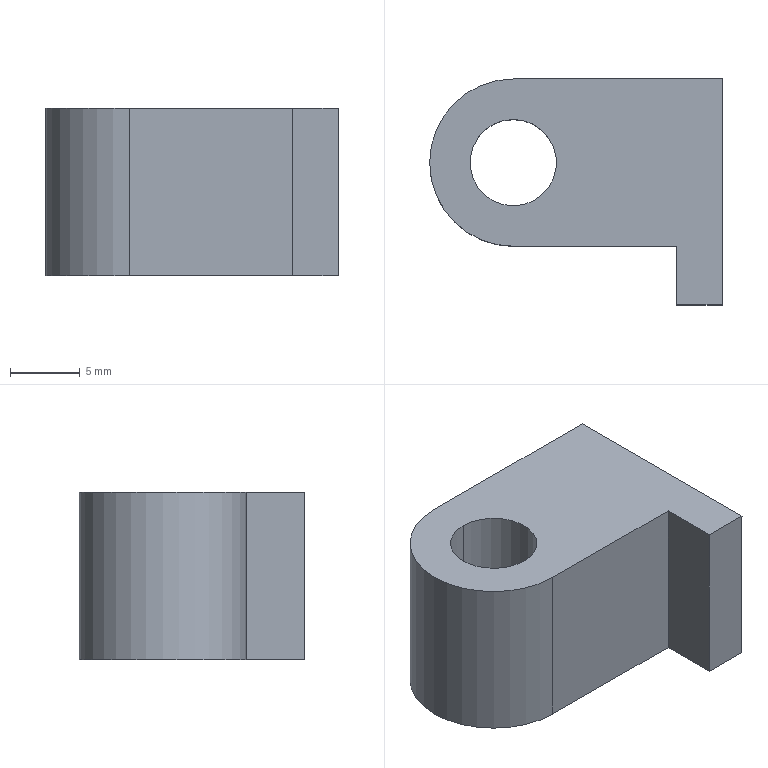Part | SolidWorks | features BaseBody 1 | 1 solid | 13 faces | box 21 x 16.2 x 12 mm | volume 2422 mm3 | plane 8 | cylinder 5 | commonest cylinder face diameters 5.3 x2 6.2 x2 12 x1
STEP:
#1=CARTESIAN_POINT('',(0.,-3.1,12.));
#2=VERTEX_POINT('',#1);
#3=CARTESIAN_POINT('',(0.,3.1,12.));
#4=VERTEX_POINT('',#3);
#5=CARTESIAN_POINT('',(0.,0.,12.));
#6=DIRECTION('',(0.,0.,-1.));
#7=DIRECTION('',(0.,1.,0.));
#8=AXIS2_PLACEMENT_3D('',#5,#6,#7);
#9=CIRCLE('',#8,3.1);
#10=EDGE_CURVE('',#2,#4,#9,.T.);
#11=ORIENTED_EDGE('',*,*,#10,.F.);
#12=CARTESIAN_POINT('',(0.,-3.1,0.));
#13=VERTEX_POINT('',#12);
#14=CARTESIAN_POINT('',(0.,-3.1,12.));
#15=DIRECTION('',(0.,0.,-1.));
#16=VECTOR('',#15,1000.);
#17=LINE('',#14,#16);
#18=EDGE_CURVE('',#2,#13,#17,.T.);
#19=ORIENTED_EDGE('',*,*,#18,.T.);
#20=CARTESIAN_POINT('',(0.,3.1,0.));
#21=VERTEX_POINT('',#20);
#22=CARTESIAN_POINT('',(0.,0.,0.));
#23=DIRECTION('',(0.,0.,1.));
#24=DIRECTION('',(0.,1.,0.));
#25=AXIS2_PLACEMENT_3D('',#22,#23,#24);
#26=CIRCLE('',#25,3.1);
#27=EDGE_CURVE('',#21,#13,#26,.T.);
#28=ORIENTED_EDGE('',*,*,#27,.F.);
#29=CARTESIAN_POINT('',(0.,3.1,12.));
#30=DIRECTION('',(0.,0.,-1.));
#31=VECTOR('',#30,1000.);
#32=LINE('',#29,#31);
#33=EDGE_CURVE('',#4,#21,#32,.T.);
#34=ORIENTED_EDGE('',*,*,#33,.F.);
#35=EDGE_LOOP('',(#11,#19,#28,#34));
#36=FACE_OUTER_BOUND('',#35,.T.);
#37=CARTESIAN_POINT('',(0.,0.,12.));
#38=DIRECTION('',(0.,0.,-1.));
#39=DIRECTION('',(0.,1.,0.));
#40=AXIS2_PLACEMENT_3D('',#37,#38,#39);
#41=CYLINDRICAL_SURFACE('',#40,3.1);
#42=ADVANCED_FACE('',(#36),#41,.F.);
#43=CARTESIAN_POINT('',(5.,-4.75,6.));
#44=VERTEX_POINT('',#43);
#45=CARTESIAN_POINT('',(5.,0.55,6.));
#46=VERTEX_POINT('',#45);
#47=CARTESIAN_POINT('',(5.,-2.1,6.));
#48=DIRECTION('',(1.,0.,0.));
#49=DIRECTION('',(0.,1.,0.));
#50=AXIS2_PLACEMENT_3D('',#47,#48,#49);
#51=CIRCLE('',#50,2.65);
#52=EDGE_CURVE('',#44,#46,#51,.T.);
#53=ORIENTED_EDGE('',*,*,#52,.F.);
#54=CARTESIAN_POINT('',(15.,-4.75,6.));
#55=VERTEX_POINT('',#54);
#56=CARTESIAN_POINT('',(5.,-4.75,6.));
#57=DIRECTION('',(1.,0.,0.));
#58=VECTOR('',#57,1000.);
#59=LINE('',#56,#58);
#60=EDGE_CURVE('',#44,#55,#59,.T.);
#61=ORIENTED_EDGE('',*,*,#60,.T.);
#62=CARTESIAN_POINT('',(15.,0.55,6.));
#63=VERTEX_POINT('',#62);
#64=CARTESIAN_POINT('',(15.,-2.1,6.));
#65=DIRECTION('',(1.,0.,0.));
#66=DIRECTION('',(0.,1.,0.));
#67=AXIS2_PLACEMENT_3D('',#64,#65,#66);
#68=CIRCLE('',#67,2.65);
#69=EDGE_CURVE('',#55,#63,#68,.T.);
#70=ORIENTED_EDGE('',*,*,#69,.T.);
#71=CARTESIAN_POINT('',(5.,0.55,6.));
#72=DIRECTION('',(1.,0.,0.));
#73=VECTOR('',#72,1000.);
#74=LINE('',#71,#73);
#75=EDGE_CURVE('',#46,#63,#74,.T.);
#76=ORIENTED_EDGE('',*,*,#75,.F.);
#77=EDGE_LOOP('',(#53,#61,#70,#76));
#78=FACE_OUTER_BOUND('',#77,.T.);
#79=CARTESIAN_POINT('',(5.,-2.1,6.));
#80=DIRECTION('',(1.,0.,0.));
#81=DIRECTION('',(0.,1.,0.));
#82=AXIS2_PLACEMENT_3D('',#79,#80,#81);
#83=CYLINDRICAL_SURFACE('',#82,2.65);
#84=ADVANCED_FACE('',(#78),#83,.F.);
#85=CARTESIAN_POINT('',(0.,0.,12.));
#86=DIRECTION('',(0.,0.,-1.));
#87=DIRECTION('',(0.,1.,0.));
#88=AXIS2_PLACEMENT_3D('',#85,#86,#87);
#89=CIRCLE('',#88,3.1);
#90=EDGE_CURVE('',#4,#2,#89,.T.);
#91=ORIENTED_EDGE('',*,*,#90,.T.);
#92=ORIENTED_EDGE('',*,*,#10,.T.);
#93=EDGE_LOOP('',(#91,#92));
#94=FACE_BOUND('',#93,.T.);
#95=CARTESIAN_POINT('',(15.,-10.2,12.));
#96=VERTEX_POINT('',#95);
#97=CARTESIAN_POINT('',(15.,6.,12.));
#98=VERTEX_POINT('',#97);
#99=CARTESIAN_POINT('',(15.,0.,12.));
#100=DIRECTION('',(0.,1.,0.));
#101=VECTOR('',#100,1000.);
#102=LINE('',#99,#101);
#103=EDGE_CURVE('',#96,#98,#102,.T.);
#104=ORIENTED_EDGE('',*,*,#103,.T.);
#105=CARTESIAN_POINT('',(0.,6.,12.));
#106=VERTEX_POINT('',#105);
#107=CARTESIAN_POINT('',(0.,6.,12.));
#108=DIRECTION('',(-1.,0.,0.));
#109=VECTOR('',#108,1000.);
#110=LINE('',#107,#109);
#111=EDGE_CURVE('',#98,#106,#110,.T.);
#112=ORIENTED_EDGE('',*,*,#111,.T.);
#113=CARTESIAN_POINT('',(0.,-6.,12.));
#114=VERTEX_POINT('',#113);
#115=CARTESIAN_POINT('',(0.,0.,12.));
#116=DIRECTION('',(0.,0.,1.));
#117=DIRECTION('',(0.,1.,0.));
#118=AXIS2_PLACEMENT_3D('',#115,#116,#117);
#119=CIRCLE('',#118,6.);
#120=EDGE_CURVE('',#106,#114,#119,.T.);
#121=ORIENTED_EDGE('',*,*,#120,.T.);
#122=CARTESIAN_POINT('',(11.7,-6.,12.));
#123=VERTEX_POINT('',#122);
#124=CARTESIAN_POINT('',(0.,-6.,12.));
#125=DIRECTION('',(1.,0.,0.));
#126=VECTOR('',#125,1000.);
#127=LINE('',#124,#126);
#128=EDGE_CURVE('',#114,#123,#127,.T.);
#129=ORIENTED_EDGE('',*,*,#128,.T.);
#130=CARTESIAN_POINT('',(11.7,-10.2,12.));
#131=VERTEX_POINT('',#130);
#132=CARTESIAN_POINT('',(11.7,0.,12.));
#133=DIRECTION('',(0.,-1.,0.));
#134=VECTOR('',#133,1000.);
#135=LINE('',#132,#134);
#136=EDGE_CURVE('',#123,#131,#135,.T.);
#137=ORIENTED_EDGE('',*,*,#136,.T.);
#138=CARTESIAN_POINT('',(0.,-10.2,12.));
#139=DIRECTION('',(1.,0.,0.));
#140=VECTOR('',#139,1000.);
#141=LINE('',#138,#140);
#142=EDGE_CURVE('',#131,#96,#141,.T.);
#143=ORIENTED_EDGE('',*,*,#142,.T.);
#144=EDGE_LOOP('',(#104,#112,#121,#129,#137,#143));
#145=FACE_OUTER_BOUND('',#144,.T.);
#146=CARTESIAN_POINT('',(0.,0.,12.));
#147=DIRECTION('',(0.,0.,1.));
#148=DIRECTION('',(0.,-1.,0.));
#149=AXIS2_PLACEMENT_3D('',#146,#147,#148);
#150=PLANE('',#149);
#151=ADVANCED_FACE('',(#94,#145),#150,.T.);
#152=ORIENTED_EDGE('',*,*,#18,.F.);
#153=ORIENTED_EDGE('',*,*,#90,.F.);
#154=ORIENTED_EDGE('',*,*,#33,.T.);
#155=CARTESIAN_POINT('',(0.,0.,0.));
#156=DIRECTION('',(0.,0.,1.));
#157=DIRECTION('',(0.,1.,0.));
#158=AXIS2_PLACEMENT_3D('',#155,#156,#157);
#159=CIRCLE('',#158,3.1);
#160=EDGE_CURVE('',#13,#21,#159,.T.);
#161=ORIENTED_EDGE('',*,*,#160,.F.);
#162=EDGE_LOOP('',(#152,#153,#154,#161));
#163=FACE_OUTER_BOUND('',#162,.T.);
#164=CARTESIAN_POINT('',(0.,0.,12.));
#165=DIRECTION('',(0.,0.,-1.));
#166=DIRECTION('',(0.,1.,0.));
#167=AXIS2_PLACEMENT_3D('',#164,#165,#166);
#168=CYLINDRICAL_SURFACE('',#167,3.1);
#169=ADVANCED_FACE('',(#163),#168,.F.);
#170=CARTESIAN_POINT('',(0.,6.,0.));
#171=VERTEX_POINT('',#170);
#172=CARTESIAN_POINT('',(0.,6.,12.));
#173=DIRECTION('',(0.,0.,-1.));
#174=VECTOR('',#173,1000.);
#175=LINE('',#172,#174);
#176=EDGE_CURVE('',#106,#171,#175,.T.);
#177=ORIENTED_EDGE('',*,*,#176,.F.);
#178=ORIENTED_EDGE('',*,*,#111,.F.);
#179=CARTESIAN_POINT('',(15.,6.,0.));
#180=VERTEX_POINT('',#179);
#181=CARTESIAN_POINT('',(15.,6.,12.));
#182=DIRECTION('',(0.,0.,1.));
#183=VECTOR('',#182,1000.);
#184=LINE('',#181,#183);
#185=EDGE_CURVE('',#180,#98,#184,.T.);
#186=ORIENTED_EDGE('',*,*,#185,.F.);
#187=CARTESIAN_POINT('',(0.,6.,0.));
#188=DIRECTION('',(1.,0.,0.));
#189=VECTOR('',#188,1000.);
#190=LINE('',#187,#189);
#191=EDGE_CURVE('',#171,#180,#190,.T.);
#192=ORIENTED_EDGE('',*,*,#191,.F.);
#193=EDGE_LOOP('',(#177,#178,#186,#192));
#194=FACE_OUTER_BOUND('',#193,.T.);
#195=CARTESIAN_POINT('',(0.,6.,12.));
#196=DIRECTION('',(0.,-1.,0.));
#197=DIRECTION('',(1.,0.,0.));
#198=AXIS2_PLACEMENT_3D('',#195,#196,#197);
#199=PLANE('',#198);
#200=ADVANCED_FACE('',(#194),#199,.F.);
#201=ORIENTED_EDGE('',*,*,#185,.T.);
#202=ORIENTED_EDGE('',*,*,#103,.F.);
#203=CARTESIAN_POINT('',(15.,-10.2,0.));
#204=VERTEX_POINT('',#203);
#205=CARTESIAN_POINT('',(15.,-10.2,12.));
#206=DIRECTION('',(0.,0.,1.));
#207=VECTOR('',#206,1000.);
#208=LINE('',#205,#207);
#209=EDGE_CURVE('',#204,#96,#208,.T.);
#210=ORIENTED_EDGE('',*,*,#209,.F.);
#211=CARTESIAN_POINT('',(15.,6.,0.));
#212=DIRECTION('',(0.,-1.,0.));
#213=VECTOR('',#212,1000.);
#214=LINE('',#211,#213);
#215=EDGE_CURVE('',#180,#204,#214,.T.);
#216=ORIENTED_EDGE('',*,*,#215,.F.);
#217=EDGE_LOOP('',(#201,#202,#210,#216));
#218=FACE_OUTER_BOUND('',#217,.T.);
#219=CARTESIAN_POINT('',(15.,-2.1,6.));
#220=DIRECTION('',(1.,0.,0.));
#221=DIRECTION('',(0.,1.,0.));
#222=AXIS2_PLACEMENT_3D('',#219,#220,#221);
#223=CIRCLE('',#222,2.65);
#224=EDGE_CURVE('',#63,#55,#223,.T.);
#225=ORIENTED_EDGE('',*,*,#224,.F.);
#226=ORIENTED_EDGE('',*,*,#69,.F.);
#227=EDGE_LOOP('',(#225,#226));
#228=FACE_BOUND('',#227,.T.);
#229=CARTESIAN_POINT('',(15.,6.,12.));
#230=DIRECTION('',(-1.,0.,0.));
#231=DIRECTION('',(0.,-1.,0.));
#232=AXIS2_PLACEMENT_3D('',#229,#230,#231);
#233=PLANE('',#232);
#234=ADVANCED_FACE('',(#218,#228),#233,.F.);
#235=ORIENTED_EDGE('',*,*,#209,.T.);
#236=ORIENTED_EDGE('',*,*,#142,.F.);
#237=CARTESIAN_POINT('',(11.7,-10.2,0.));
#238=VERTEX_POINT('',#237);
#239=CARTESIAN_POINT('',(11.7,-10.2,12.));
#240=DIRECTION('',(0.,0.,1.));
#241=VECTOR('',#240,1000.);
#242=LINE('',#239,#241);
#243=EDGE_CURVE('',#238,#131,#242,.T.);
#244=ORIENTED_EDGE('',*,*,#243,.F.);
#245=CARTESIAN_POINT('',(15.,-10.2,0.));
#246=DIRECTION('',(-1.,0.,0.));
#247=VECTOR('',#246,1000.);
#248=LINE('',#245,#247);
#249=EDGE_CURVE('',#204,#238,#248,.T.);
#250=ORIENTED_EDGE('',*,*,#249,.F.);
#251=EDGE_LOOP('',(#235,#236,#244,#250));
#252=FACE_OUTER_BOUND('',#251,.T.);
#253=CARTESIAN_POINT('',(15.,-10.2,12.));
#254=DIRECTION('',(0.,1.,0.));
#255=DIRECTION('',(0.,0.,1.));
#256=AXIS2_PLACEMENT_3D('',#253,#254,#255);
#257=PLANE('',#256);
#258=ADVANCED_FACE('',(#252),#257,.F.);
#259=ORIENTED_EDGE('',*,*,#243,.T.);
#260=ORIENTED_EDGE('',*,*,#136,.F.);
#261=CARTESIAN_POINT('',(11.7,-6.,0.));
#262=VERTEX_POINT('',#261);
#263=CARTESIAN_POINT('',(11.7,-6.,12.));
#264=DIRECTION('',(0.,0.,1.));
#265=VECTOR('',#264,1000.);
#266=LINE('',#263,#265);
#267=EDGE_CURVE('',#262,#123,#266,.T.);
#268=ORIENTED_EDGE('',*,*,#267,.F.);
#269=CARTESIAN_POINT('',(11.7,-10.2,0.));
#270=DIRECTION('',(0.,1.,0.));
#271=VECTOR('',#270,1000.);
#272=LINE('',#269,#271);
#273=EDGE_CURVE('',#238,#262,#272,.T.);
#274=ORIENTED_EDGE('',*,*,#273,.F.);
#275=EDGE_LOOP('',(#259,#260,#268,#274));
#276=FACE_OUTER_BOUND('',#275,.T.);
#277=CARTESIAN_POINT('',(11.7,-10.2,12.));
#278=DIRECTION('',(1.,0.,0.));
#279=DIRECTION('',(0.,0.,-1.));
#280=AXIS2_PLACEMENT_3D('',#277,#278,#279);
#281=PLANE('',#280);
#282=ADVANCED_FACE('',(#276),#281,.F.);
#283=ORIENTED_EDGE('',*,*,#267,.T.);
#284=ORIENTED_EDGE('',*,*,#128,.F.);
#285=CARTESIAN_POINT('',(0.,-6.,0.));
#286=VERTEX_POINT('',#285);
#287=CARTESIAN_POINT('',(0.,-6.,12.));
#288=DIRECTION('',(0.,0.,1.));
#289=VECTOR('',#288,1000.);
#290=LINE('',#287,#289);
#291=EDGE_CURVE('',#286,#114,#290,.T.);
#292=ORIENTED_EDGE('',*,*,#291,.F.);
#293=CARTESIAN_POINT('',(11.7,-6.,0.));
#294=DIRECTION('',(-1.,0.,0.));
#295=VECTOR('',#294,1000.);
#296=LINE('',#293,#295);
#297=EDGE_CURVE('',#262,#286,#296,.T.);
#298=ORIENTED_EDGE('',*,*,#297,.F.);
#299=EDGE_LOOP('',(#283,#284,#292,#298));
#300=FACE_OUTER_BOUND('',#299,.T.);
#301=CARTESIAN_POINT('',(11.7,-6.,12.));
#302=DIRECTION('',(0.,1.,0.));
#303=DIRECTION('',(-1.,0.,0.));
#304=AXIS2_PLACEMENT_3D('',#301,#302,#303);
#305=PLANE('',#304);
#306=ADVANCED_FACE('',(#300),#305,.F.);
#307=CARTESIAN_POINT('',(0.,0.,0.));
#308=DIRECTION('',(0.,0.,1.));
#309=DIRECTION('',(0.,1.,0.));
#310=AXIS2_PLACEMENT_3D('',#307,#308,#309);
#311=CIRCLE('',#310,6.);
#312=EDGE_CURVE('',#171,#286,#311,.T.);
#313=ORIENTED_EDGE('',*,*,#312,.T.);
#314=ORIENTED_EDGE('',*,*,#291,.T.);
#315=ORIENTED_EDGE('',*,*,#120,.F.);
#316=ORIENTED_EDGE('',*,*,#176,.T.);
#317=EDGE_LOOP('',(#313,#314,#315,#316));
#318=FACE_OUTER_BOUND('',#317,.T.);
#319=CARTESIAN_POINT('',(0.,0.,12.));
#320=DIRECTION('',(0.,0.,-1.));
#321=DIRECTION('',(0.,1.,0.));
#322=AXIS2_PLACEMENT_3D('',#319,#320,#321);
#323=CYLINDRICAL_SURFACE('',#322,6.);
#324=ADVANCED_FACE('',(#318),#323,.T.);
#325=ORIENTED_EDGE('',*,*,#27,.T.);
#326=ORIENTED_EDGE('',*,*,#160,.T.);
#327=EDGE_LOOP('',(#325,#326));
#328=FACE_BOUND('',#327,.T.);
#329=ORIENTED_EDGE('',*,*,#191,.T.);
#330=ORIENTED_EDGE('',*,*,#215,.T.);
#331=ORIENTED_EDGE('',*,*,#249,.T.);
#332=ORIENTED_EDGE('',*,*,#273,.T.);
#333=ORIENTED_EDGE('',*,*,#297,.T.);
#334=ORIENTED_EDGE('',*,*,#312,.F.);
#335=EDGE_LOOP('',(#329,#330,#331,#332,#333,#334));
#336=FACE_OUTER_BOUND('',#335,.T.);
#337=CARTESIAN_POINT('',(0.,0.,0.));
#338=DIRECTION('',(0.,0.,1.));
#339=DIRECTION('',(0.,-1.,0.));
#340=AXIS2_PLACEMENT_3D('',#337,#338,#339);
#341=PLANE('',#340);
#342=ADVANCED_FACE('',(#328,#336),#341,.F.);
#343=ORIENTED_EDGE('',*,*,#60,.F.);
#344=CARTESIAN_POINT('',(5.,-2.1,6.));
#345=DIRECTION('',(1.,0.,0.));
#346=DIRECTION('',(0.,1.,0.));
#347=AXIS2_PLACEMENT_3D('',#344,#345,#346);
#348=CIRCLE('',#347,2.65);
#349=EDGE_CURVE('',#46,#44,#348,.T.);
#350=ORIENTED_EDGE('',*,*,#349,.F.);
#351=ORIENTED_EDGE('',*,*,#75,.T.);
#352=ORIENTED_EDGE('',*,*,#224,.T.);
#353=EDGE_LOOP('',(#343,#350,#351,#352));
#354=FACE_OUTER_BOUND('',#353,.T.);
#355=CARTESIAN_POINT('',(5.,-2.1,6.));
#356=DIRECTION('',(1.,0.,0.));
#357=DIRECTION('',(0.,1.,0.));
#358=AXIS2_PLACEMENT_3D('',#355,#356,#357);
#359=CYLINDRICAL_SURFACE('',#358,2.65);
#360=ADVANCED_FACE('',(#354),#359,.F.);
#361=ORIENTED_EDGE('',*,*,#349,.T.);
#362=ORIENTED_EDGE('',*,*,#52,.T.);
#363=EDGE_LOOP('',(#361,#362));
#364=FACE_OUTER_BOUND('',#363,.T.);
#365=CARTESIAN_POINT('',(5.,-2.1,6.));
#366=DIRECTION('',(1.,0.,0.));
#367=DIRECTION('',(0.,1.,0.));
#368=AXIS2_PLACEMENT_3D('',#365,#366,#367);
#369=PLANE('',#368);
#370=ADVANCED_FACE('',(#364),#369,.T.);
#371=CLOSED_SHELL('',(#42,#84,#151,#169,#200,#234,#258,#282,#306,#324,#342,#360,#370));
#372=MANIFOLD_SOLID_BREP('',#371);
#373=CARTESIAN_POINT('',(0.,0.,0.));
#374=DIRECTION('',(0.,0.,1.));
#375=DIRECTION('',(1.,0.,0.));
#376=AXIS2_PLACEMENT_3D('',#373,#374,#375);
#377=(LENGTH_UNIT()NAMED_UNIT(*)SI_UNIT(.MILLI.,.METRE.));
#378=UNCERTAINTY_MEASURE_WITH_UNIT(LENGTH_MEASURE(0.00001),#377,'','');
#379=(NAMED_UNIT(*)PLANE_ANGLE_UNIT()SI_UNIT($,.RADIAN.));
#380=(NAMED_UNIT(*)SI_UNIT($,.STERADIAN.)SOLID_ANGLE_UNIT());
#381=(GEOMETRIC_REPRESENTATION_CONTEXT(3)GLOBAL_UNCERTAINTY_ASSIGNED_CONTEXT((#378))GLOBAL_UNIT_ASSIGNED_CONTEXT((#377,#379,#380))REPRESENTATION_CONTEXT('',''));
#382=ADVANCED_BREP_SHAPE_REPRESENTATION('',(#372,#376),#381);